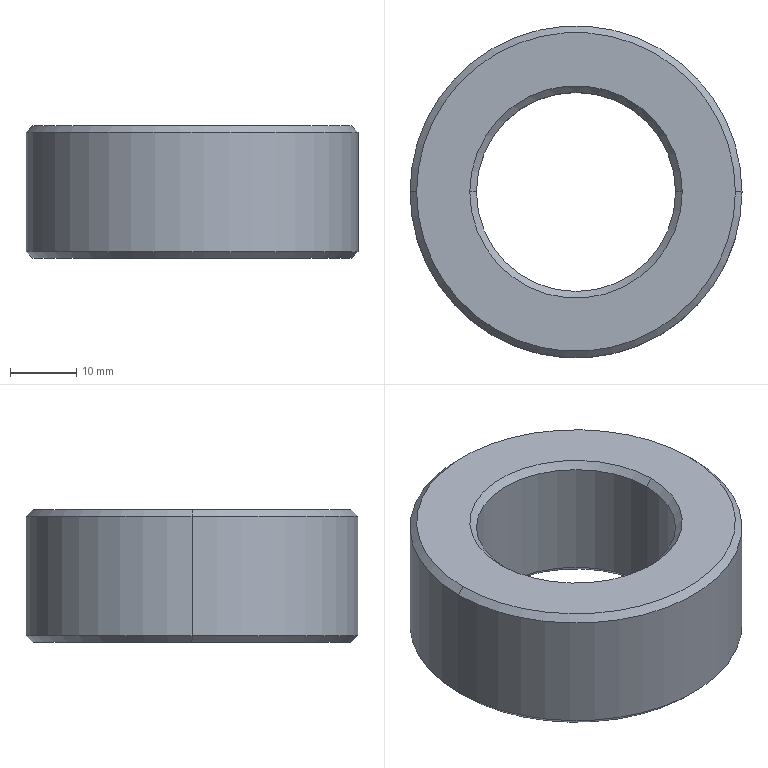Part | SolidWorks | features Chamfer 1, Extrusion 1 | 1 solid | 14 faces | box 50 x 50 x 20 mm | volume 24881 mm3 | cone 8 | cylinder 4 | plane 2 | commonest cylinder face diameters 30 x2 50 x2
STEP:
#1=CARTESIAN_POINT('',(24.,0.,20.));
#2=VERTEX_POINT('',#1);
#3=CARTESIAN_POINT('',(-24.,0.,20.));
#4=VERTEX_POINT('',#3);
#5=CARTESIAN_POINT('',(0.,0.,20.));
#6=DIRECTION('',(0.,0.,1.));
#7=DIRECTION('',(1.,0.,0.));
#8=AXIS2_PLACEMENT_3D('',#5,#6,#7);
#9=CIRCLE('',#8,24.);
#10=EDGE_CURVE('',#2,#4,#9,.T.);
#11=ORIENTED_EDGE('',*,*,#10,.F.);
#12=CARTESIAN_POINT('',(25.,0.,19.));
#13=VERTEX_POINT('',#12);
#14=CARTESIAN_POINT('',(24.,0.,20.));
#15=DIRECTION('',(0.7071,0.,-0.7071));
#16=VECTOR('',#15,1000.);
#17=LINE('',#14,#16);
#18=EDGE_CURVE('',#2,#13,#17,.T.);
#19=ORIENTED_EDGE('',*,*,#18,.T.);
#20=CARTESIAN_POINT('',(-25.,0.,19.));
#21=VERTEX_POINT('',#20);
#22=CARTESIAN_POINT('',(0.,0.,19.));
#23=DIRECTION('',(0.,0.,-1.));
#24=DIRECTION('',(1.,0.,0.));
#25=AXIS2_PLACEMENT_3D('',#22,#23,#24);
#26=CIRCLE('',#25,25.);
#27=EDGE_CURVE('',#21,#13,#26,.T.);
#28=ORIENTED_EDGE('',*,*,#27,.F.);
#29=CARTESIAN_POINT('',(-24.,0.,20.));
#30=DIRECTION('',(-0.7071,0.,-0.7071));
#31=VECTOR('',#30,1000.);
#32=LINE('',#29,#31);
#33=EDGE_CURVE('',#4,#21,#32,.T.);
#34=ORIENTED_EDGE('',*,*,#33,.F.);
#35=EDGE_LOOP('',(#11,#19,#28,#34));
#36=FACE_OUTER_BOUND('',#35,.T.);
#37=CARTESIAN_POINT('',(0.,0.,20.));
#38=DIRECTION('',(0.,0.,-1.));
#39=DIRECTION('',(-1.,0.,0.));
#40=AXIS2_PLACEMENT_3D('',#37,#38,#39);
#41=CONICAL_SURFACE('',#40,24.,0.7854);
#42=ADVANCED_FACE('',(#36),#41,.T.);
#43=CARTESIAN_POINT('',(-24.,0.,0.));
#44=VERTEX_POINT('',#43);
#45=CARTESIAN_POINT('',(24.,0.,0.));
#46=VERTEX_POINT('',#45);
#47=CARTESIAN_POINT('',(0.,0.,0.));
#48=DIRECTION('',(0.,0.,-1.));
#49=DIRECTION('',(1.,0.,0.));
#50=AXIS2_PLACEMENT_3D('',#47,#48,#49);
#51=CIRCLE('',#50,24.);
#52=EDGE_CURVE('',#44,#46,#51,.T.);
#53=ORIENTED_EDGE('',*,*,#52,.F.);
#54=CARTESIAN_POINT('',(-25.,0.,1.));
#55=VERTEX_POINT('',#54);
#56=CARTESIAN_POINT('',(-25.,0.,1.));
#57=DIRECTION('',(-0.7071,0.,0.7071));
#58=VECTOR('',#57,1000.);
#59=LINE('',#56,#58);
#60=EDGE_CURVE('',#44,#55,#59,.T.);
#61=ORIENTED_EDGE('',*,*,#60,.T.);
#62=CARTESIAN_POINT('',(25.,0.,1.));
#63=VERTEX_POINT('',#62);
#64=CARTESIAN_POINT('',(0.,0.,1.));
#65=DIRECTION('',(0.,0.,1.));
#66=DIRECTION('',(1.,0.,0.));
#67=AXIS2_PLACEMENT_3D('',#64,#65,#66);
#68=CIRCLE('',#67,25.);
#69=EDGE_CURVE('',#63,#55,#68,.T.);
#70=ORIENTED_EDGE('',*,*,#69,.F.);
#71=CARTESIAN_POINT('',(25.,0.,1.));
#72=DIRECTION('',(0.7071,0.,0.7071));
#73=VECTOR('',#72,1000.);
#74=LINE('',#71,#73);
#75=EDGE_CURVE('',#46,#63,#74,.T.);
#76=ORIENTED_EDGE('',*,*,#75,.F.);
#77=EDGE_LOOP('',(#53,#61,#70,#76));
#78=FACE_OUTER_BOUND('',#77,.T.);
#79=CARTESIAN_POINT('',(0.,0.,1.));
#80=DIRECTION('',(0.,0.,1.));
#81=DIRECTION('',(1.,0.,0.));
#82=AXIS2_PLACEMENT_3D('',#79,#80,#81);
#83=CONICAL_SURFACE('',#82,25.,0.7854);
#84=ADVANCED_FACE('',(#78),#83,.T.);
#85=CARTESIAN_POINT('',(-15.,0.,19.));
#86=VERTEX_POINT('',#85);
#87=CARTESIAN_POINT('',(15.,0.,19.));
#88=VERTEX_POINT('',#87);
#89=CARTESIAN_POINT('',(0.,0.,19.));
#90=DIRECTION('',(0.,0.,1.));
#91=DIRECTION('',(1.,0.,0.));
#92=AXIS2_PLACEMENT_3D('',#89,#90,#91);
#93=CIRCLE('',#92,15.);
#94=EDGE_CURVE('',#86,#88,#93,.T.);
#95=ORIENTED_EDGE('',*,*,#94,.F.);
#96=CARTESIAN_POINT('',(-16.,0.,20.));
#97=VERTEX_POINT('',#96);
#98=CARTESIAN_POINT('',(-15.,0.,19.));
#99=DIRECTION('',(-0.7071,0.,0.7071));
#100=VECTOR('',#99,1000.);
#101=LINE('',#98,#100);
#102=EDGE_CURVE('',#86,#97,#101,.T.);
#103=ORIENTED_EDGE('',*,*,#102,.T.);
#104=CARTESIAN_POINT('',(16.,0.,20.));
#105=VERTEX_POINT('',#104);
#106=CARTESIAN_POINT('',(0.,0.,20.));
#107=DIRECTION('',(0.,0.,-1.));
#108=DIRECTION('',(1.,0.,0.));
#109=AXIS2_PLACEMENT_3D('',#106,#107,#108);
#110=CIRCLE('',#109,16.);
#111=EDGE_CURVE('',#105,#97,#110,.T.);
#112=ORIENTED_EDGE('',*,*,#111,.F.);
#113=CARTESIAN_POINT('',(15.,0.,19.));
#114=DIRECTION('',(0.7071,0.,0.7071));
#115=VECTOR('',#114,1000.);
#116=LINE('',#113,#115);
#117=EDGE_CURVE('',#88,#105,#116,.T.);
#118=ORIENTED_EDGE('',*,*,#117,.F.);
#119=EDGE_LOOP('',(#95,#103,#112,#118));
#120=FACE_OUTER_BOUND('',#119,.T.);
#121=CARTESIAN_POINT('',(0.,0.,19.));
#122=DIRECTION('',(0.,0.,1.));
#123=DIRECTION('',(1.,0.,0.));
#124=AXIS2_PLACEMENT_3D('',#121,#122,#123);
#125=CONICAL_SURFACE('',#124,15.,0.7854);
#126=ADVANCED_FACE('',(#120),#125,.F.);
#127=CARTESIAN_POINT('',(15.,0.,1.));
#128=VERTEX_POINT('',#127);
#129=CARTESIAN_POINT('',(-15.,0.,1.));
#130=VERTEX_POINT('',#129);
#131=CARTESIAN_POINT('',(0.,0.,1.));
#132=DIRECTION('',(0.,0.,-1.));
#133=DIRECTION('',(1.,0.,0.));
#134=AXIS2_PLACEMENT_3D('',#131,#132,#133);
#135=CIRCLE('',#134,15.);
#136=EDGE_CURVE('',#128,#130,#135,.T.);
#137=ORIENTED_EDGE('',*,*,#136,.F.);
#138=CARTESIAN_POINT('',(16.,0.,0.));
#139=VERTEX_POINT('',#138);
#140=CARTESIAN_POINT('',(16.,0.,0.));
#141=DIRECTION('',(0.7071,0.,-0.7071));
#142=VECTOR('',#141,1000.);
#143=LINE('',#140,#142);
#144=EDGE_CURVE('',#128,#139,#143,.T.);
#145=ORIENTED_EDGE('',*,*,#144,.T.);
#146=CARTESIAN_POINT('',(-16.,0.,0.));
#147=VERTEX_POINT('',#146);
#148=CARTESIAN_POINT('',(0.,0.,0.));
#149=DIRECTION('',(0.,0.,1.));
#150=DIRECTION('',(1.,0.,0.));
#151=AXIS2_PLACEMENT_3D('',#148,#149,#150);
#152=CIRCLE('',#151,16.);
#153=EDGE_CURVE('',#147,#139,#152,.T.);
#154=ORIENTED_EDGE('',*,*,#153,.F.);
#155=CARTESIAN_POINT('',(-16.,0.,0.));
#156=DIRECTION('',(-0.7071,0.,-0.7071));
#157=VECTOR('',#156,1000.);
#158=LINE('',#155,#157);
#159=EDGE_CURVE('',#130,#147,#158,.T.);
#160=ORIENTED_EDGE('',*,*,#159,.F.);
#161=EDGE_LOOP('',(#137,#145,#154,#160));
#162=FACE_OUTER_BOUND('',#161,.T.);
#163=CARTESIAN_POINT('',(0.,0.,0.));
#164=DIRECTION('',(0.,0.,-1.));
#165=DIRECTION('',(-1.,0.,0.));
#166=AXIS2_PLACEMENT_3D('',#163,#164,#165);
#167=CONICAL_SURFACE('',#166,16.,0.7854);
#168=ADVANCED_FACE('',(#162),#167,.F.);
#169=ORIENTED_EDGE('',*,*,#94,.T.);
#170=CARTESIAN_POINT('',(15.,0.,20.));
#171=DIRECTION('',(0.,0.,-1.));
#172=VECTOR('',#171,1000.);
#173=LINE('',#170,#172);
#174=EDGE_CURVE('',#88,#128,#173,.T.);
#175=ORIENTED_EDGE('',*,*,#174,.T.);
#176=ORIENTED_EDGE('',*,*,#136,.T.);
#177=CARTESIAN_POINT('',(-15.,0.,20.));
#178=DIRECTION('',(0.,0.,-1.));
#179=VECTOR('',#178,1000.);
#180=LINE('',#177,#179);
#181=EDGE_CURVE('',#86,#130,#180,.T.);
#182=ORIENTED_EDGE('',*,*,#181,.F.);
#183=EDGE_LOOP('',(#169,#175,#176,#182));
#184=FACE_OUTER_BOUND('',#183,.T.);
#185=CARTESIAN_POINT('',(0.,0.,20.));
#186=DIRECTION('',(0.,0.,-1.));
#187=DIRECTION('',(-1.,0.,0.));
#188=AXIS2_PLACEMENT_3D('',#185,#186,#187);
#189=CYLINDRICAL_SURFACE('',#188,15.);
#190=ADVANCED_FACE('',(#184),#189,.F.);
#191=ORIENTED_EDGE('',*,*,#27,.T.);
#192=CARTESIAN_POINT('',(25.,0.,20.));
#193=DIRECTION('',(0.,0.,-1.));
#194=VECTOR('',#193,1000.);
#195=LINE('',#192,#194);
#196=EDGE_CURVE('',#13,#63,#195,.T.);
#197=ORIENTED_EDGE('',*,*,#196,.T.);
#198=ORIENTED_EDGE('',*,*,#69,.T.);
#199=CARTESIAN_POINT('',(-25.,0.,20.));
#200=DIRECTION('',(0.,0.,-1.));
#201=VECTOR('',#200,1000.);
#202=LINE('',#199,#201);
#203=EDGE_CURVE('',#21,#55,#202,.T.);
#204=ORIENTED_EDGE('',*,*,#203,.F.);
#205=EDGE_LOOP('',(#191,#197,#198,#204));
#206=FACE_OUTER_BOUND('',#205,.T.);
#207=CARTESIAN_POINT('',(0.,0.,20.));
#208=DIRECTION('',(0.,0.,-1.));
#209=DIRECTION('',(-1.,0.,0.));
#210=AXIS2_PLACEMENT_3D('',#207,#208,#209);
#211=CYLINDRICAL_SURFACE('',#210,25.);
#212=ADVANCED_FACE('',(#206),#211,.T.);
#213=ORIENTED_EDGE('',*,*,#111,.T.);
#214=CARTESIAN_POINT('',(0.,0.,20.));
#215=DIRECTION('',(0.,0.,-1.));
#216=DIRECTION('',(1.,0.,0.));
#217=AXIS2_PLACEMENT_3D('',#214,#215,#216);
#218=CIRCLE('',#217,16.);
#219=EDGE_CURVE('',#97,#105,#218,.T.);
#220=ORIENTED_EDGE('',*,*,#219,.T.);
#221=EDGE_LOOP('',(#213,#220));
#222=FACE_BOUND('',#221,.T.);
#223=CARTESIAN_POINT('',(0.,0.,20.));
#224=DIRECTION('',(0.,0.,1.));
#225=DIRECTION('',(1.,0.,0.));
#226=AXIS2_PLACEMENT_3D('',#223,#224,#225);
#227=CIRCLE('',#226,24.);
#228=EDGE_CURVE('',#4,#2,#227,.T.);
#229=ORIENTED_EDGE('',*,*,#228,.T.);
#230=ORIENTED_EDGE('',*,*,#10,.T.);
#231=EDGE_LOOP('',(#229,#230));
#232=FACE_OUTER_BOUND('',#231,.T.);
#233=CARTESIAN_POINT('',(0.,0.,20.));
#234=DIRECTION('',(0.,0.,1.));
#235=DIRECTION('',(1.,0.,0.));
#236=AXIS2_PLACEMENT_3D('',#233,#234,#235);
#237=PLANE('',#236);
#238=ADVANCED_FACE('',(#222,#232),#237,.T.);
#239=ORIENTED_EDGE('',*,*,#153,.T.);
#240=CARTESIAN_POINT('',(0.,0.,0.));
#241=DIRECTION('',(0.,0.,1.));
#242=DIRECTION('',(1.,0.,0.));
#243=AXIS2_PLACEMENT_3D('',#240,#241,#242);
#244=CIRCLE('',#243,16.);
#245=EDGE_CURVE('',#139,#147,#244,.T.);
#246=ORIENTED_EDGE('',*,*,#245,.T.);
#247=EDGE_LOOP('',(#239,#246));
#248=FACE_BOUND('',#247,.T.);
#249=CARTESIAN_POINT('',(0.,0.,0.));
#250=DIRECTION('',(0.,0.,-1.));
#251=DIRECTION('',(1.,0.,0.));
#252=AXIS2_PLACEMENT_3D('',#249,#250,#251);
#253=CIRCLE('',#252,24.);
#254=EDGE_CURVE('',#46,#44,#253,.T.);
#255=ORIENTED_EDGE('',*,*,#254,.T.);
#256=ORIENTED_EDGE('',*,*,#52,.T.);
#257=EDGE_LOOP('',(#255,#256));
#258=FACE_OUTER_BOUND('',#257,.T.);
#259=CARTESIAN_POINT('',(0.,0.,0.));
#260=DIRECTION('',(0.,0.,1.));
#261=DIRECTION('',(1.,0.,0.));
#262=AXIS2_PLACEMENT_3D('',#259,#260,#261);
#263=PLANE('',#262);
#264=ADVANCED_FACE('',(#248,#258),#263,.F.);
#265=ORIENTED_EDGE('',*,*,#196,.F.);
#266=CARTESIAN_POINT('',(0.,0.,19.));
#267=DIRECTION('',(0.,0.,-1.));
#268=DIRECTION('',(1.,0.,0.));
#269=AXIS2_PLACEMENT_3D('',#266,#267,#268);
#270=CIRCLE('',#269,25.);
#271=EDGE_CURVE('',#13,#21,#270,.T.);
#272=ORIENTED_EDGE('',*,*,#271,.T.);
#273=ORIENTED_EDGE('',*,*,#203,.T.);
#274=CARTESIAN_POINT('',(0.,0.,1.));
#275=DIRECTION('',(0.,0.,1.));
#276=DIRECTION('',(1.,0.,0.));
#277=AXIS2_PLACEMENT_3D('',#274,#275,#276);
#278=CIRCLE('',#277,25.);
#279=EDGE_CURVE('',#55,#63,#278,.T.);
#280=ORIENTED_EDGE('',*,*,#279,.T.);
#281=EDGE_LOOP('',(#265,#272,#273,#280));
#282=FACE_OUTER_BOUND('',#281,.T.);
#283=CARTESIAN_POINT('',(0.,0.,20.));
#284=DIRECTION('',(0.,0.,-1.));
#285=DIRECTION('',(-1.,0.,0.));
#286=AXIS2_PLACEMENT_3D('',#283,#284,#285);
#287=CYLINDRICAL_SURFACE('',#286,25.);
#288=ADVANCED_FACE('',(#282),#287,.T.);
#289=ORIENTED_EDGE('',*,*,#174,.F.);
#290=CARTESIAN_POINT('',(0.,0.,19.));
#291=DIRECTION('',(0.,0.,1.));
#292=DIRECTION('',(1.,0.,0.));
#293=AXIS2_PLACEMENT_3D('',#290,#291,#292);
#294=CIRCLE('',#293,15.);
#295=EDGE_CURVE('',#88,#86,#294,.T.);
#296=ORIENTED_EDGE('',*,*,#295,.T.);
#297=ORIENTED_EDGE('',*,*,#181,.T.);
#298=CARTESIAN_POINT('',(0.,0.,1.));
#299=DIRECTION('',(0.,0.,-1.));
#300=DIRECTION('',(1.,0.,0.));
#301=AXIS2_PLACEMENT_3D('',#298,#299,#300);
#302=CIRCLE('',#301,15.);
#303=EDGE_CURVE('',#130,#128,#302,.T.);
#304=ORIENTED_EDGE('',*,*,#303,.T.);
#305=EDGE_LOOP('',(#289,#296,#297,#304));
#306=FACE_OUTER_BOUND('',#305,.T.);
#307=CARTESIAN_POINT('',(0.,0.,20.));
#308=DIRECTION('',(0.,0.,-1.));
#309=DIRECTION('',(-1.,0.,0.));
#310=AXIS2_PLACEMENT_3D('',#307,#308,#309);
#311=CYLINDRICAL_SURFACE('',#310,15.);
#312=ADVANCED_FACE('',(#306),#311,.F.);
#313=ORIENTED_EDGE('',*,*,#144,.F.);
#314=ORIENTED_EDGE('',*,*,#303,.F.);
#315=ORIENTED_EDGE('',*,*,#159,.T.);
#316=ORIENTED_EDGE('',*,*,#245,.F.);
#317=EDGE_LOOP('',(#313,#314,#315,#316));
#318=FACE_OUTER_BOUND('',#317,.T.);
#319=CARTESIAN_POINT('',(0.,0.,0.));
#320=DIRECTION('',(0.,0.,-1.));
#321=DIRECTION('',(-1.,0.,0.));
#322=AXIS2_PLACEMENT_3D('',#319,#320,#321);
#323=CONICAL_SURFACE('',#322,16.,0.7854);
#324=ADVANCED_FACE('',(#318),#323,.F.);
#325=ORIENTED_EDGE('',*,*,#102,.F.);
#326=ORIENTED_EDGE('',*,*,#295,.F.);
#327=ORIENTED_EDGE('',*,*,#117,.T.);
#328=ORIENTED_EDGE('',*,*,#219,.F.);
#329=EDGE_LOOP('',(#325,#326,#327,#328));
#330=FACE_OUTER_BOUND('',#329,.T.);
#331=CARTESIAN_POINT('',(0.,0.,19.));
#332=DIRECTION('',(0.,0.,1.));
#333=DIRECTION('',(1.,0.,0.));
#334=AXIS2_PLACEMENT_3D('',#331,#332,#333);
#335=CONICAL_SURFACE('',#334,15.,0.7854);
#336=ADVANCED_FACE('',(#330),#335,.F.);
#337=ORIENTED_EDGE('',*,*,#60,.F.);
#338=ORIENTED_EDGE('',*,*,#254,.F.);
#339=ORIENTED_EDGE('',*,*,#75,.T.);
#340=ORIENTED_EDGE('',*,*,#279,.F.);
#341=EDGE_LOOP('',(#337,#338,#339,#340));
#342=FACE_OUTER_BOUND('',#341,.T.);
#343=CARTESIAN_POINT('',(0.,0.,1.));
#344=DIRECTION('',(0.,0.,1.));
#345=DIRECTION('',(1.,0.,0.));
#346=AXIS2_PLACEMENT_3D('',#343,#344,#345);
#347=CONICAL_SURFACE('',#346,25.,0.7854);
#348=ADVANCED_FACE('',(#342),#347,.T.);
#349=ORIENTED_EDGE('',*,*,#18,.F.);
#350=ORIENTED_EDGE('',*,*,#228,.F.);
#351=ORIENTED_EDGE('',*,*,#33,.T.);
#352=ORIENTED_EDGE('',*,*,#271,.F.);
#353=EDGE_LOOP('',(#349,#350,#351,#352));
#354=FACE_OUTER_BOUND('',#353,.T.);
#355=CARTESIAN_POINT('',(0.,0.,20.));
#356=DIRECTION('',(0.,0.,-1.));
#357=DIRECTION('',(-1.,0.,0.));
#358=AXIS2_PLACEMENT_3D('',#355,#356,#357);
#359=CONICAL_SURFACE('',#358,24.,0.7854);
#360=ADVANCED_FACE('',(#354),#359,.T.);
#361=CLOSED_SHELL('',(#42,#84,#126,#168,#190,#212,#238,#264,#288,#312,#324,#336,#348,#360));
#362=MANIFOLD_SOLID_BREP('',#361);
#363=CARTESIAN_POINT('',(0.,0.,0.));
#364=DIRECTION('',(0.,0.,1.));
#365=DIRECTION('',(1.,0.,0.));
#366=AXIS2_PLACEMENT_3D('',#363,#364,#365);
#367=(LENGTH_UNIT()NAMED_UNIT(*)SI_UNIT(.MILLI.,.METRE.));
#368=UNCERTAINTY_MEASURE_WITH_UNIT(LENGTH_MEASURE(0.00001),#367,'','');
#369=(NAMED_UNIT(*)PLANE_ANGLE_UNIT()SI_UNIT($,.RADIAN.));
#370=(NAMED_UNIT(*)SI_UNIT($,.STERADIAN.)SOLID_ANGLE_UNIT());
#371=(GEOMETRIC_REPRESENTATION_CONTEXT(3)GLOBAL_UNCERTAINTY_ASSIGNED_CONTEXT((#368))GLOBAL_UNIT_ASSIGNED_CONTEXT((#367,#369,#370))REPRESENTATION_CONTEXT('',''));
#372=ADVANCED_BREP_SHAPE_REPRESENTATION('',(#362,#366),#371);